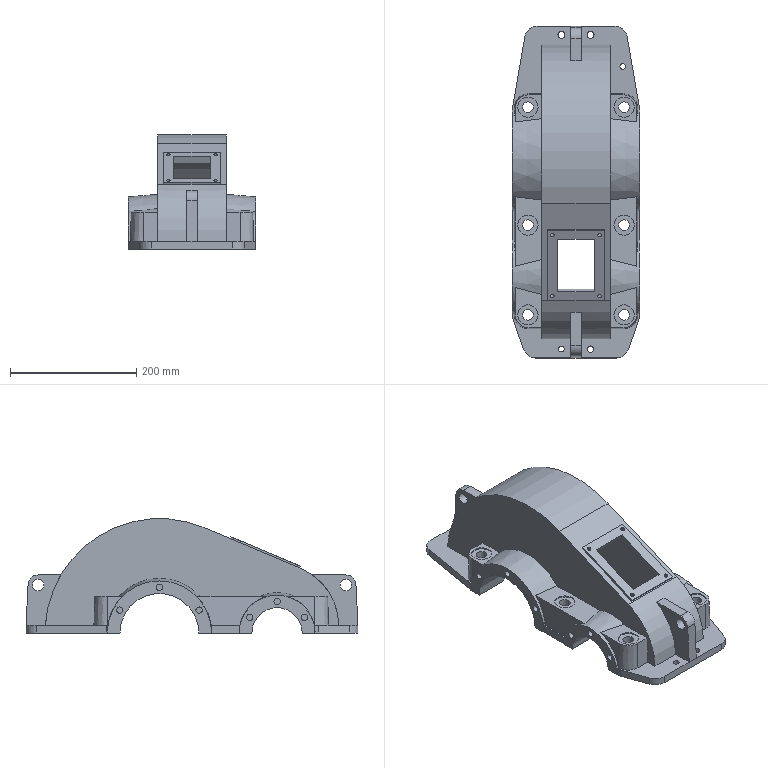Part | NX | features SIMPLE HOLE 56, DATUM_CSYS 27, HOLE PACKAGE 26, SKETCH 26, EXTRUDE 18, EXTRACT_FACE 16, EXTRACT_DATUM_AXIS 10, BLEND 8, CBORE_HOLE 7, EXTRACT_DATUM_PLANE 6, FSET 6, Instance Feature 5, Mirror Feature 5, DRAFT 4, EXTRACT_STRING 2 | 1 solid | 141 faces | box 202 x 525 x 181 mm | volume 2847836 mm3 | plane 84 | cylinder 49 | cone 8 | commonest cylinder face diameters 10 x13 32 x8 17 x6 6 x4 40 x4 9 x2